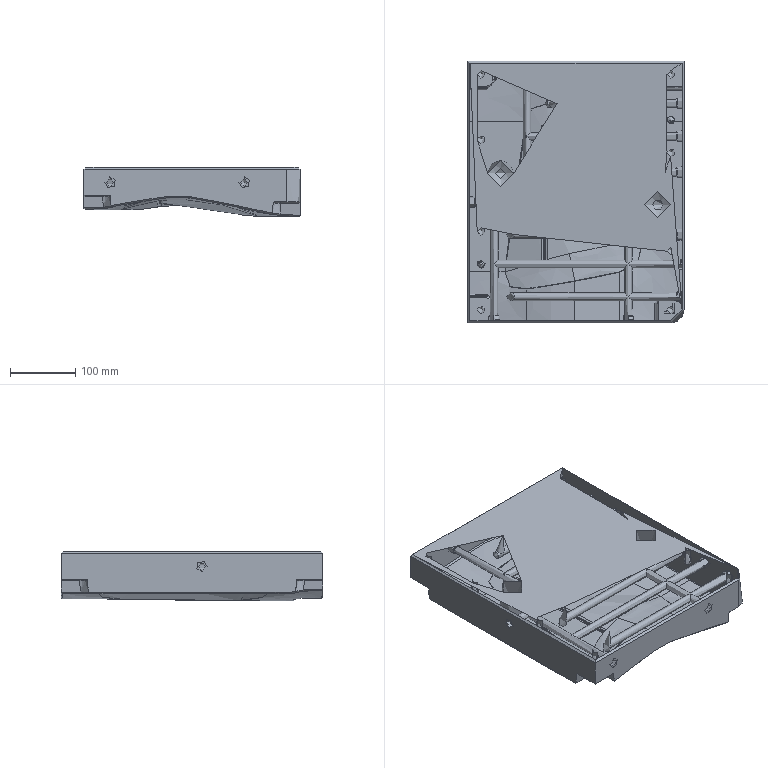Part | STEP file | P011002F001-000 | 1 solid | 1265 faces | volume 7659861 mm3 | plane 568 | other 257 | cone 201 | spline 160 | cylinder 79 | commonest cylinder face diameters 12 x37 10.2 x12 11.96 x8 4 x6 10.18 x6 24 x3